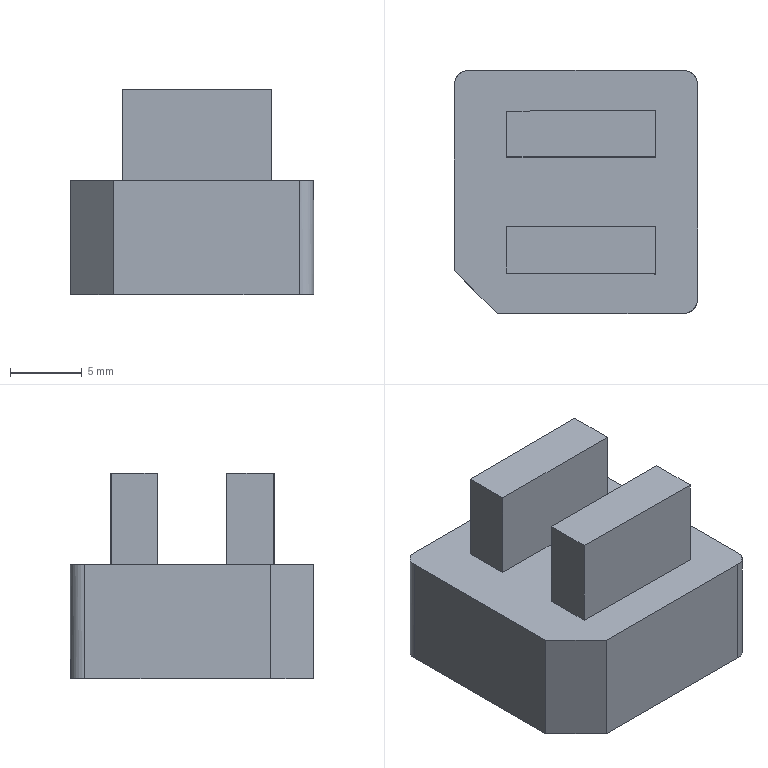NC program | PowerMill | posted with a generic post | part box 17 x 17 x 14.396 mm
Lines 1 to 1008 of 69084:
%
O0001
N104 ( POWERMILL CB  : 2026004.0)
N105 ( POST VER      : 2026.0.0.5161)
N106 ( OPTION FILE   : FANUC)
N107 ( OUTPUT WORKPLANE : WORLD)
N108 (  )
N109 ( TOOL LIST )
N110 (---------------------------------------)
N111 ( NO. | ID        | DIA.| TIP RAD|LENGTH)
N112 (---------------------------------------)
N113 (    1|D10C_1_1   |10.0 |  0.0   |69.84 )
N114 (   15|D3C_1_1    | 3.0 |  0.0   | 61.6 )
N115 (    3|D10_1_1    |10.0 |  0.0   |69.56 )
N116 (   10|D3_1_1     | 3.0 |  0.0   |61.56 )
N117 (   13|TEXT_D4_1_1| 4.0 |  0.3   |61.64 )
N118 (---------------------------------------)
N119 (  )
N120 ( NUMBER OF TOOLPATHS: 11.0 )
N121 ( ESTIMATED PROGRAM DURATION: 0 HOURS 10 MIN 28 SEC)
N122 (  )
N123 G00 G21 G80 G40 G17
N124 G90
N125 G54
N126 G53 Z0.0
N127 (---------------)
N128 ( START TOOLPATH : 精公开粗01-扫面平行-D10C )
N129 (---------------)
N130 ( TOOL NO.    :1 )
N131 ( TOOL TYPE   : ENDMILL)
N132 ( TOOL ID     : D10C_1_1)
N133 ( TOOL DIA    : 10.0 LENGTH 69.84)
N134 T1
N135 M6
N136 S8000 M03
N137 G00 G90 X0.0 Y0.0
N138 G43 Z10.2 H1
N139
N140 G05 P10000 R4
N141 X11.28 Y11.28
N142 Z1.126
N143 G01 Z-0.074 F6000.0
N144 X-11.28 F10000.0
N145 Y5.64
N146 X11.28
N147 Y0.0
N148 X-11.28
N149 Y-5.64
N150 X11.28
N151 Y-11.28
N152 X-11.28
N153 X-16.28
N154 G00 Z10.2
N155 G05 P0
N156 (---------------)
N157 ( END TOOLPATH : 精公开粗01-扫面平行-D10C )
N158 (---------------)
N159 ( START TOOLPATH : 精公开粗01-外形偏置-D10C )
N160 (---------------)
N161 G00 X0.3365 Y-0.0255 Z9.876
N162 G05 P10000 R4
N163 X-17.929 Y-10.5753
N164 Z0.6831
N165 G01 Z-0.5169 F6000.0
N166 X-17.4015 F10000.0
N167 G03 X-12.654 Y-5.8278 I0.0 J4.7475
N168 G01 Y12.468
N169 G02 X-11.654 Y13.468 I1.0 J0.0
N170 G01 X12.327
N171 G02 X13.327 Y12.468 I0.0 J-1.0
N172 G01 Y-12.519
N173 G02 X12.327 Y-13.519 I-1.0 J0.0
N174 G01 X-11.654
N175 G02 X-12.654 Y-12.519 I0.0 J1.0
N176 G01 Y-5.8278
N177 X-10.1543 Y-5.8262
N178 X-10.1562 Y-2.7325
N179 X-10.1353 Y-1.9591
N180 X-10.0077 Y-1.1856
N181 X-9.7559 Y-0.4122
N182 X-9.6387 Y-0.1635
N183 G03 X-9.6372 Y0.2593 I-0.4524 J0.213
N184 G01 X-9.6843 Y0.3612
N185 X-9.945 Y1.1346
N186 X-10.0804 Y1.9081
N187 X-10.1048 Y2.3039
N188 Y5.7609
N189 X-10.0266 Y6.5486
N190 X-9.8295 Y7.3221
N191 X-9.4981 Y8.0955
N192 X-9.3313 Y8.389
N193 X-9.0002 Y8.8689
N194 X-8.5579 Y9.3707
N195 X-8.2646 Y9.6423
N196 X-7.7845 Y10.0088
N197 X-7.0681 Y10.4158
N198 X-6.2376 Y10.7232
N199 X-5.4642 Y10.8766
N200 X-4.6908 Y10.9161
N201 X5.3638 Y10.9687
N202 X6.1372 Y10.9367
N203 X6.9106 Y10.7908
N204 X7.6841 Y10.5183
N205 X8.4575 Y10.0958
N206 X9.0488 Y9.6423
N207 X9.2309 Y9.4733
N208 X9.7637 Y8.8689
N209 X10.0043 Y8.5218
N210 X10.2482 Y8.0955
N211 X10.5695 Y7.3221
N212 X10.7578 Y6.5486
N213 X10.8275 Y5.7752
N214 X10.8281 Y2.6815
N215 X10.8024 Y1.9081
N216 X10.6669 Y1.1346
N217 X10.4063 Y0.3612
N218 X10.3359 Y0.2119
N219 G03 X10.3347 Y-0.2115 I0.4524 J-0.2131
N220 G01 X10.4278 Y-0.4122
N221 X10.6796 Y-1.1856
N222 X10.8072 Y-1.9591
N223 X10.8281 Y-2.7325
N224 X10.8274 Y-5.8262
N225 X10.7778 Y-6.4672
N226 X10.569 Y-7.3731
N227 X10.2476 Y-8.1465
N228 X10.0043 Y-8.5715
N229 X9.7627 Y-8.9199
N230 X9.2309 Y-9.523
N231 X9.0474 Y-9.6933
N232 X8.4575 Y-10.1455
N233 X7.8999 Y-10.4668
N234 X7.6841 Y-10.5681
N235 X6.9106 Y-10.8406
N236 X6.1372 Y-10.9864
N237 X5.3638 Y-11.0185
N238 X-4.6908 Y-10.9658
N239 X-5.4642 Y-10.932
N240 X-6.2376 Y-10.7863
N241 X-7.0111 Y-10.514
N242 X-7.7845 Y-10.0917
N243 X-8.3128 Y-9.6933
N244 X-8.5579 Y-9.4695
N245 X-9.0491 Y-8.9199
N246 X-9.3313 Y-8.5186
N247 X-9.5472 Y-8.1465
N248 X-9.8791 Y-7.3731
N249 X-10.0764 Y-6.5996
N250 X-10.1543 Y-5.8262
N251 X-12.654 Y-5.8278
N252 G00 Z3.2903
N253 G01 X-17.929 Y-10.5753
N254 G00 Z0.2903
N255 G01 Z-0.9097 F6000.0
N256 X-17.4015 F10000.0
N257 G03 X-12.654 Y-5.8278 I0.0 J4.7475
N258 G01 Y12.468
N259 G02 X-11.654 Y13.468 I1.0 J0.0
N260 G01 X12.327
N261 G02 X13.327 Y12.468 I0.0 J-1.0
N262 G01 Y-12.519
N263 G02 X12.327 Y-13.519 I-1.0 J0.0
N264 G01 X-11.654
N265 G02 X-12.654 Y-12.519 I0.0 J1.0
N266 G01 Y-5.8278
N267 X-10.1543 Y-5.8262
N268 X-10.1563 Y-2.7325
N269 X-10.1353 Y-1.9591
N270 X-10.0077 Y-1.1856
N271 X-9.7559 Y-0.4122
N272 X-9.6388 Y-0.1635
N273 G03 X-9.6372 Y0.2593 I-0.4523 J0.213
N274 G01 X-9.6843 Y0.3612
N275 X-9.945 Y1.1346
N276 X-10.0804 Y1.9081
N277 X-10.1048 Y2.3039
N278 Y5.7609
N279 X-10.0266 Y6.5486
N280 X-9.8296 Y7.3221
N281 X-9.4981 Y8.0955
N282 X-9.3313 Y8.389
N283 X-9.0002 Y8.8689
N284 X-8.5579 Y9.3707
N285 X-8.2646 Y9.6423
N286 X-7.7845 Y10.0088
N287 X-7.0681 Y10.4158
N288 X-6.2376 Y10.7232
N289 X-5.4642 Y10.8766
N290 X-4.6908 Y10.9161
N291 X5.3638 Y10.9687
N292 X6.1372 Y10.9367
N293 X6.9106 Y10.7908
N294 X7.6841 Y10.5183
N295 X8.4575 Y10.0958
N296 X9.0489 Y9.6423
N297 X9.2309 Y9.4733
N298 X9.7637 Y8.8689
N299 X10.0043 Y8.5218
N300 X10.2482 Y8.0955
N301 X10.5695 Y7.3221
N302 X10.7578 Y6.5486
N303 X10.8275 Y5.7752
N304 X10.8281 Y2.6815
N305 X10.8024 Y1.9081
N306 X10.6669 Y1.1346
N307 X10.4063 Y0.3612
N308 X10.3359 Y0.2119
N309 G03 X10.3347 Y-0.2116 I0.4524 J-0.2131
N310 G01 X10.4278 Y-0.4122
N311 X10.6796 Y-1.1856
N312 X10.8072 Y-1.9591
N313 X10.8281 Y-2.7325
N314 X10.8274 Y-5.8262
N315 X10.7778 Y-6.4672
N316 X10.569 Y-7.3731
N317 X10.2476 Y-8.1465
N318 X10.0043 Y-8.5715
N319 X9.7627 Y-8.9199
N320 X9.2309 Y-9.523
N321 X9.0474 Y-9.6933
N322 X8.4575 Y-10.1455
N323 X7.8999 Y-10.4668
N324 X7.6841 Y-10.5681
N325 X6.9106 Y-10.8406
N326 X6.1372 Y-10.9864
N327 X5.3638 Y-11.0185
N328 X-4.6908 Y-10.9658
N329 X-5.4642 Y-10.932
N330 X-6.2376 Y-10.7863
N331 X-7.0111 Y-10.514
N332 X-7.7845 Y-10.0917
N333 X-8.3128 Y-9.6933
N334 X-8.5579 Y-9.4695
N335 X-9.0491 Y-8.9199
N336 X-9.3313 Y-8.5186
N337 X-9.5472 Y-8.1465
N338 X-9.8791 Y-7.3731
N339 X-10.0764 Y-6.5996
N340 X-10.1543 Y-5.8262
N341 X-12.654 Y-5.8278
N342 G00 Z2.8974
N343 G01 X-17.929 Y-10.5753
N344 G00 Z-0.1026
N345 G01 Z-1.3026 F6000.0
N346 X-17.4015 F10000.0
N347 G03 X-12.654 Y-5.8278 I0.0 J4.7475
N348 G01 Y12.468
N349 G02 X-11.654 Y13.468 I1.0 J0.0
N350 G01 X12.327
N351 G02 X13.327 Y12.468 I0.0 J-1.0
N352 G01 Y-12.519
N353 G02 X12.327 Y-13.519 I-1.0 J0.0
N354 G01 X-11.654
N355 G02 X-12.654 Y-12.519 I0.0 J1.0
N356 G01 Y-5.8278
N357 X-10.1543 Y-5.8262
N358 X-10.1563 Y-2.7325
N359 X-10.1353 Y-1.9591
N360 X-10.0077 Y-1.1856
N361 X-9.7559 Y-0.4122
N362 X-9.6388 Y-0.1635
N363 G03 X-9.6372 Y0.2593 I-0.4523 J0.213
N364 G01 X-9.6844 Y0.3612
N365 X-9.945 Y1.1346
N366 X-10.0804 Y1.9081
N367 X-10.1048 Y2.3039
N368 Y5.7609
N369 X-10.0267 Y6.5486
N370 X-9.8296 Y7.3221
N371 X-9.4981 Y8.0955
N372 X-9.3313 Y8.389
N373 X-9.0002 Y8.8689
N374 X-8.5579 Y9.3707
N375 X-8.2646 Y9.6423
N376 X-7.7845 Y10.0088
N377 X-7.0681 Y10.4158
N378 X-6.2376 Y10.7232
N379 X-5.4642 Y10.8766
N380 X-4.6908 Y10.9161
N381 X5.3638 Y10.9687
N382 X6.1372 Y10.9367
N383 X6.9106 Y10.7908
N384 X7.6841 Y10.5183
N385 X8.4575 Y10.0958
N386 X9.0489 Y9.6423
N387 X9.2309 Y9.4733
N388 X9.7637 Y8.8689
N389 X10.0043 Y8.5218
N390 X10.2482 Y8.0955
N391 X10.5695 Y7.3221
N392 X10.7578 Y6.5486
N393 X10.8275 Y5.7752
N394 X10.8281 Y2.6815
N395 X10.8024 Y1.9081
N396 X10.6669 Y1.1346
N397 X10.4063 Y0.3612
N398 X10.336 Y0.2119
N399 G03 X10.3347 Y-0.2116 I0.4523 J-0.2131
N400 G01 X10.4278 Y-0.4122
N401 X10.6796 Y-1.1856
N402 X10.8072 Y-1.9591
N403 X10.8281 Y-2.7325
N404 X10.8274 Y-5.8262
N405 X10.7778 Y-6.4672
N406 X10.569 Y-7.3731
N407 X10.2476 Y-8.1465
N408 X10.0043 Y-8.5715
N409 X9.7627 Y-8.9199
N410 X9.2309 Y-9.523
N411 X9.0474 Y-9.6933
N412 X8.4575 Y-10.1455
N413 X7.8999 Y-10.4668
N414 X7.6841 Y-10.5681
N415 X6.9106 Y-10.8406
N416 X6.1372 Y-10.9864
N417 X5.3638 Y-11.0185
N418 X-4.6908 Y-10.9658
N419 X-5.4642 Y-10.932
N420 X-6.2376 Y-10.7863
N421 X-7.0111 Y-10.514
N422 X-7.7845 Y-10.0917
N423 X-8.3128 Y-9.6933
N424 X-8.5579 Y-9.4695
N425 X-9.0491 Y-8.9199
N426 X-9.3313 Y-8.5186
N427 X-9.5472 Y-8.1465
N428 X-9.8791 Y-7.3731
N429 X-10.0764 Y-6.5996
N430 X-10.1543 Y-5.8262
N431 X-12.654 Y-5.8278
N432 G00 Z2.5045
N433 G01 X-17.929 Y-10.5753
N434 G00 Z-0.4955
N435 G01 Z-1.6955 F6000.0
N436 X-17.4015 F10000.0
N437 G03 X-12.654 Y-5.8278 I0.0 J4.7475
N438 G01 Y12.468
N439 G02 X-11.654 Y13.468 I1.0 J0.0
N440 G01 X12.327
N441 G02 X13.327 Y12.468 I0.0 J-1.0
N442 G01 Y-12.519
N443 G02 X12.327 Y-13.519 I-1.0 J0.0
N444 G01 X-11.654
N445 G02 X-12.654 Y-12.519 I0.0 J1.0
N446 G01 Y-5.8278
N447 X-10.1543 Y-5.8262
N448 X-10.1563 Y-2.7325
N449 X-10.1353 Y-1.9591
N450 X-10.0077 Y-1.1856
N451 X-9.7559 Y-0.4122
N452 X-9.6388 Y-0.1635
N453 G03 X-9.6372 Y0.2593 I-0.4523 J0.213
N454 G01 X-9.6844 Y0.3612
N455 X-9.945 Y1.1346
N456 X-10.0804 Y1.9081
N457 X-10.1048 Y2.3039
N458 Y5.7609
N459 X-10.0267 Y6.5486
N460 X-9.8296 Y7.3221
N461 X-9.4981 Y8.0955
N462 X-9.3313 Y8.389
N463 X-9.0002 Y8.8689
N464 X-8.5579 Y9.3707
N465 X-8.2646 Y9.6423
N466 X-7.7845 Y10.0088
N467 X-7.0681 Y10.4158
N468 X-6.2376 Y10.7232
N469 X-5.4642 Y10.8767
N470 X-4.6908 Y10.9161
N471 X5.3638 Y10.9687
N472 X6.1372 Y10.9367
N473 X6.9106 Y10.7908
N474 X7.6841 Y10.5183
N475 X8.4575 Y10.0958
N476 X9.0489 Y9.6423
N477 X9.2309 Y9.4733
N478 X9.7637 Y8.8689
N479 X10.0043 Y8.5218
N480 X10.2482 Y8.0955
N481 X10.5695 Y7.3221
N482 X10.7578 Y6.5486
N483 X10.8275 Y5.7752
N484 X10.8281 Y2.6815
N485 X10.8024 Y1.9081
N486 X10.667 Y1.1346
N487 X10.4063 Y0.3612
N488 X10.336 Y0.2119
N489 G03 X10.3347 Y-0.2116 I0.4523 J-0.2131
N490 G01 X10.4278 Y-0.4122
N491 X10.6796 Y-1.1856
N492 X10.8072 Y-1.9591
N493 X10.8281 Y-2.7325
N494 X10.8274 Y-5.8262
N495 X10.7778 Y-6.4672
N496 X10.569 Y-7.3731
N497 X10.2476 Y-8.1465
N498 X10.0043 Y-8.5715
N499 X9.7627 Y-8.9199
N500 X9.2309 Y-9.523
N501 X9.0475 Y-9.6933
N502 X8.4575 Y-10.1456
N503 X7.8999 Y-10.4668
N504 X7.6841 Y-10.5681
N505 X6.9106 Y-10.8406
N506 X6.1372 Y-10.9864
N507 X5.3638 Y-11.0185
N508 X-4.6908 Y-10.9658
N509 X-5.4642 Y-10.932
N510 X-6.2376 Y-10.7863
N511 X-7.0111 Y-10.514
N512 X-7.7845 Y-10.0917
N513 X-8.3128 Y-9.6933
N514 X-8.5579 Y-9.4695
N515 X-9.0491 Y-8.9199
N516 X-9.3313 Y-8.5187
N517 X-9.5472 Y-8.1465
N518 X-9.8791 Y-7.3731
N519 X-10.0764 Y-6.5996
N520 X-10.1543 Y-5.8262
N521 X-12.654 Y-5.8278
N522 G00 Z2.1116
N523 G01 X-17.929 Y-10.5753
N524 G00 Z-0.8884
N525 G01 Z-2.0884 F6000.0
N526 X-17.4015 F10000.0
N527 G03 X-12.654 Y-5.8278 I0.0 J4.7475
N528 G01 Y12.468
N529 G02 X-11.654 Y13.468 I1.0 J0.0
N530 G01 X12.327
N531 G02 X13.327 Y12.468 I0.0 J-1.0
N532 G01 Y-12.519
N533 G02 X12.327 Y-13.519 I-1.0 J0.0
N534 G01 X-11.654
N535 G02 X-12.654 Y-12.519 I0.0 J1.0
N536 G01 Y-5.8278
N537 X-10.1543 Y-5.8262
N538 X-10.1563 Y-2.7325
N539 X-10.1353 Y-1.9591
N540 X-10.0077 Y-1.1856
N541 X-9.7559 Y-0.4122
N542 X-9.6388 Y-0.1635
N543 G03 X-9.6372 Y0.2593 I-0.4523 J0.213
N544 G01 X-9.6844 Y0.3612
N545 X-9.945 Y1.1346
N546 X-10.0804 Y1.9081
N547 X-10.1048 Y2.3038
N548 Y5.7609
N549 X-10.0267 Y6.5486
N550 X-9.8296 Y7.3221
N551 X-9.4981 Y8.0955
N552 X-9.3313 Y8.389
N553 X-9.0002 Y8.8689
N554 X-8.5579 Y9.3707
N555 X-8.2646 Y9.6423
N556 X-7.7845 Y10.0088
N557 X-7.0681 Y10.4158
N558 X-6.2376 Y10.7232
N559 X-5.4642 Y10.8767
N560 X-4.6908 Y10.9161
N561 X5.3638 Y10.9687
N562 X6.1372 Y10.9367
N563 X6.9106 Y10.7908
N564 X7.6841 Y10.5183
N565 X8.4575 Y10.0958
N566 X9.0489 Y9.6423
N567 X9.2309 Y9.4733
N568 X9.7637 Y8.8689
N569 X10.0043 Y8.5218
N570 X10.2482 Y8.0955
N571 X10.5695 Y7.3221
N572 X10.7578 Y6.5486
N573 X10.8275 Y5.7752
N574 X10.8281 Y2.6815
N575 X10.8024 Y1.9081
N576 X10.667 Y1.1346
N577 X10.4063 Y0.3612
N578 X10.336 Y0.2119
N579 G03 X10.3347 Y-0.2116 I0.4523 J-0.2131
N580 G01 X10.4278 Y-0.4122
N581 X10.6796 Y-1.1856
N582 X10.8072 Y-1.9591
N583 X10.8281 Y-2.7325
N584 X10.8274 Y-5.8262
N585 X10.7778 Y-6.4672
N586 X10.569 Y-7.3731
N587 X10.2476 Y-8.1465
N588 X10.0043 Y-8.5715
N589 X9.7627 Y-8.9199
N590 X9.2309 Y-9.523
N591 X9.0475 Y-9.6933
N592 X8.4575 Y-10.1456
N593 X7.8999 Y-10.4668
N594 X7.6841 Y-10.5681
N595 X6.9106 Y-10.8406
N596 X6.1372 Y-10.9864
N597 X5.3638 Y-11.0185
N598 X-4.6908 Y-10.9658
N599 X-5.4642 Y-10.932
N600 X-6.2376 Y-10.7863
N601 X-7.0111 Y-10.514
N602 X-7.7845 Y-10.0917
N603 X-8.3128 Y-9.6933
N604 X-8.5579 Y-9.4695
N605 X-9.0491 Y-8.9199
N606 X-9.3313 Y-8.5187
N607 X-9.5472 Y-8.1465
N608 X-9.8791 Y-7.3731
N609 X-10.0764 Y-6.5996
N610 X-10.1543 Y-5.8262
N611 X-12.654 Y-5.8278
N612 G00 Z1.7188
N613 G01 X-17.929 Y-10.5753
N614 G00 Z-1.2813
N615 G01 Z-2.4813 F6000.0
N616 X-17.4015 F10000.0
N617 G03 X-12.654 Y-5.8278 I0.0 J4.7475
N618 G01 Y12.468
N619 G02 X-11.654 Y13.468 I1.0 J0.0
N620 G01 X12.327
N621 G02 X13.327 Y12.468 I0.0 J-1.0
N622 G01 Y-12.519
N623 G02 X12.327 Y-13.519 I-1.0 J0.0
N624 G01 X-11.654
N625 G02 X-12.654 Y-12.519 I0.0 J1.0
N626 G01 Y-5.8278
N627 X-10.1543 Y-5.8262
N628 X-10.1563 Y-2.7325
N629 X-10.1353 Y-1.9591
N630 X-10.0077 Y-1.1856
N631 X-9.7559 Y-0.4122
N632 X-9.6388 Y-0.1635
N633 G03 X-9.6373 Y0.2593 I-0.4523 J0.213
N634 G01 X-9.6844 Y0.3612
N635 X-9.945 Y1.1346
N636 X-10.0804 Y1.9081
N637 X-10.1048 Y2.3038
N638 Y5.7609
N639 X-10.0267 Y6.5486
N640 X-9.8296 Y7.3221
N641 X-9.4981 Y8.0955
N642 X-9.3313 Y8.389
N643 X-9.0002 Y8.8689
N644 X-8.5579 Y9.3707
N645 X-8.2646 Y9.6423
N646 X-7.7845 Y10.0088
N647 X-7.0681 Y10.4158
N648 X-6.2376 Y10.7232
N649 X-5.4642 Y10.8767
N650 X-4.6908 Y10.9161
N651 X5.3638 Y10.9688
N652 X6.1372 Y10.9367
N653 X6.9106 Y10.7908
N654 X7.6841 Y10.5183
N655 X8.4575 Y10.0958
N656 X9.0489 Y9.6423
N657 X9.2309 Y9.4733
N658 X9.7637 Y8.8689
N659 X10.0043 Y8.5218
N660 X10.2483 Y8.0955
N661 X10.5695 Y7.3221
N662 X10.7578 Y6.5486
N663 X10.8275 Y5.7752
N664 X10.8282 Y2.6815
N665 X10.8024 Y1.9081
N666 X10.667 Y1.1346
N667 X10.4063 Y0.3612
N668 X10.336 Y0.2119
N669 G03 X10.3347 Y-0.2116 I0.4523 J-0.2131
N670 G01 X10.4278 Y-0.4122
N671 X10.6797 Y-1.1856
N672 X10.8072 Y-1.9591
N673 X10.8282 Y-2.7325
N674 X10.8274 Y-5.8262
N675 X10.7778 Y-6.4672
N676 X10.569 Y-7.3731
N677 X10.2476 Y-8.1465
N678 X10.0043 Y-8.5716
N679 X9.7627 Y-8.9199
N680 X9.2309 Y-9.523
N681 X9.0475 Y-9.6933
N682 X8.4575 Y-10.1456
N683 X7.8999 Y-10.4668
N684 X7.6841 Y-10.5681
N685 X6.9106 Y-10.8406
N686 X6.1372 Y-10.9864
N687 X5.3638 Y-11.0185
N688 X-4.6908 Y-10.9658
N689 X-5.4642 Y-10.932
N690 X-6.2376 Y-10.7863
N691 X-7.0111 Y-10.514
N692 X-7.7845 Y-10.0917
N693 X-8.3128 Y-9.6933
N694 X-8.5579 Y-9.4695
N695 X-9.0491 Y-8.9199
N696 X-9.3313 Y-8.5187
N697 X-9.5472 Y-8.1465
N698 X-9.8791 Y-7.3731
N699 X-10.0764 Y-6.5996
N700 X-10.1543 Y-5.8262
N701 X-12.654 Y-5.8278
N702 G00 Z1.3259
N703 G01 X-17.929 Y-10.5753
N704 G00 Z-1.6741
N705 G01 Z-2.8741 F6000.0
N706 X-17.4015 F10000.0
N707 G03 X-12.654 Y-5.8278 I0.0 J4.7475
N708 G01 Y12.468
N709 G02 X-11.654 Y13.468 I1.0 J0.0
N710 G01 X12.327
N711 G02 X13.327 Y12.468 I0.0 J-1.0
N712 G01 Y-12.519
N713 G02 X12.327 Y-13.519 I-1.0 J0.0
N714 G01 X-11.654
N715 G02 X-12.654 Y-12.519 I0.0 J1.0
N716 G01 Y-5.8278
N717 X-10.1543 Y-5.8262
N718 X-10.1563 Y-2.7325
N719 X-10.1353 Y-1.9591
N720 X-10.0077 Y-1.1856
N721 X-9.7559 Y-0.4122
N722 X-9.6388 Y-0.1635
N723 G03 X-9.6373 Y0.2593 I-0.4523 J0.213
N724 G01 X-9.6844 Y0.3612
N725 X-9.945 Y1.1346
N726 X-10.0804 Y1.9081
N727 X-10.1048 Y2.3038
N728 Y5.7609
N729 X-10.0267 Y6.5486
N730 X-9.8296 Y7.3221
N731 X-9.4981 Y8.0955
N732 X-9.3313 Y8.389
N733 X-9.0002 Y8.8689
N734 X-8.5579 Y9.3708
N735 X-8.2646 Y9.6423
N736 X-7.7845 Y10.0088
N737 X-7.0681 Y10.4158
N738 X-6.2376 Y10.7232
N739 X-5.4642 Y10.8767
N740 X-4.6908 Y10.9161
N741 X5.3638 Y10.9688
N742 X6.1372 Y10.9367
N743 X6.9106 Y10.7908
N744 X7.6841 Y10.5183
N745 X8.4575 Y10.0958
N746 X9.0489 Y9.6423
N747 X9.2309 Y9.4733
N748 X9.7637 Y8.8689
N749 X10.0043 Y8.5218
N750 X10.2483 Y8.0955
N751 X10.5695 Y7.3221
N752 X10.7579 Y6.5486
N753 X10.8275 Y5.7752
N754 X10.8282 Y2.6815
N755 X10.8024 Y1.9081
N756 X10.667 Y1.1346
N757 X10.4063 Y0.3612
N758 X10.336 Y0.212
N759 G03 X10.3347 Y-0.2116 I0.4523 J-0.2132
N760 G01 X10.4278 Y-0.4122
N761 X10.6797 Y-1.1856
N762 X10.8072 Y-1.9591
N763 X10.8282 Y-2.7325
N764 X10.8274 Y-5.8262
N765 X10.7778 Y-6.4672
N766 X10.569 Y-7.3731
N767 X10.2476 Y-8.1465
N768 X10.0043 Y-8.5716
N769 X9.7627 Y-8.9199
N770 X9.2309 Y-9.523
N771 X9.0475 Y-9.6933
N772 X8.4575 Y-10.1456
N773 X7.8999 Y-10.4668
N774 X7.6841 Y-10.5681
N775 X6.9106 Y-10.8406
N776 X6.1372 Y-10.9864
N777 X5.3638 Y-11.0185
N778 X-4.6908 Y-10.9658
N779 X-5.4642 Y-10.932
N780 X-6.2376 Y-10.7863
N781 X-7.0111 Y-10.514
N782 X-7.7845 Y-10.0917
N783 X-8.3128 Y-9.6933
N784 X-8.5579 Y-9.4695
N785 X-9.0491 Y-8.9199
N786 X-9.3313 Y-8.5187
N787 X-9.5472 Y-8.1465
N788 X-9.8791 Y-7.3731
N789 X-10.0764 Y-6.5996
N790 X-10.1543 Y-5.8262
N791 X-12.654 Y-5.8278
N792 G00 Z0.933
N793 G01 X-17.929 Y-10.5753
N794 G00 Z-2.067
N795 G01 Z-3.267 F6000.0
N796 X-17.4015 F10000.0
N797 G03 X-12.654 Y-5.8278 I0.0 J4.7475
N798 G01 Y12.468
N799 G02 X-11.654 Y13.468 I1.0 J0.0
N800 G01 X12.327
N801 G02 X13.327 Y12.468 I0.0 J-1.0
N802 G01 Y-12.519
N803 G02 X12.327 Y-13.519 I-1.0 J0.0
N804 G01 X-11.654
N805 G02 X-12.654 Y-12.519 I0.0 J1.0
N806 G01 Y-5.8278
N807 X-10.1543 Y-5.8262
N808 X-10.1563 Y-2.7325
N809 X-10.1353 Y-1.9591
N810 X-10.0077 Y-1.1856
N811 X-9.7559 Y-0.4122
N812 X-9.6388 Y-0.1635
N813 G03 X-9.6373 Y0.2593 I-0.4523 J0.213
N814 G01 X-9.6844 Y0.3612
N815 X-9.945 Y1.1346
N816 X-10.0804 Y1.9081
N817 X-10.1048 Y2.3038
N818 Y5.7609
N819 X-10.0267 Y6.5486
N820 X-9.8296 Y7.3221
N821 X-9.4981 Y8.0955
N822 X-9.3313 Y8.389
N823 X-9.0002 Y8.8689
N824 X-8.5579 Y9.3708
N825 X-8.2646 Y9.6423
N826 X-7.7845 Y10.0088
N827 X-7.0681 Y10.4158
N828 X-6.2376 Y10.7232
N829 X-5.4642 Y10.8767
N830 X-4.6908 Y10.9162
N831 X5.3638 Y10.9688
N832 X6.1372 Y10.9367
N833 X6.9106 Y10.7908
N834 X7.6841 Y10.5184
N835 X8.4575 Y10.0958
N836 X9.0489 Y9.6423
N837 X9.2309 Y9.4733
N838 X9.7637 Y8.8689
N839 X10.0043 Y8.5218
N840 X10.2483 Y8.0955
N841 X10.5695 Y7.3221
N842 X10.7579 Y6.5486
N843 X10.8275 Y5.7752
N844 X10.8282 Y2.6815
N845 X10.8024 Y1.9081
N846 X10.667 Y1.1346
N847 X10.4063 Y0.3612
N848 X10.336 Y0.212
N849 G03 X10.3347 Y-0.2116 I0.4523 J-0.2132
N850 G01 X10.4278 Y-0.4122
N851 X10.6797 Y-1.1856
N852 X10.8072 Y-1.9591
N853 X10.8282 Y-2.7325
N854 X10.8274 Y-5.8262
N855 X10.7778 Y-6.4672
N856 X10.569 Y-7.3731
N857 X10.2476 Y-8.1465
N858 X10.0043 Y-8.5716
N859 X9.7627 Y-8.9199
N860 X9.2309 Y-9.523
N861 X9.0475 Y-9.6933
N862 X8.4575 Y-10.1456
N863 X7.8999 Y-10.4668
N864 X7.6841 Y-10.5681
N865 X6.9106 Y-10.8406
N866 X6.1372 Y-10.9864
N867 X5.3638 Y-11.0185
N868 X-4.6908 Y-10.9658
N869 X-5.4642 Y-10.932
N870 X-6.2376 Y-10.7863
N871 X-7.0111 Y-10.514
N872 X-7.7845 Y-10.0917
N873 X-8.3128 Y-9.6933
N874 X-8.5579 Y-9.4695
N875 X-9.0491 Y-8.9199
N876 X-9.3313 Y-8.5187
N877 X-9.5473 Y-8.1465
N878 X-9.8791 Y-7.3731
N879 X-10.0764 Y-6.5996
N880 X-10.1543 Y-5.8262
N881 X-12.654 Y-5.8278
N882 G00 Z0.5401
N883 G01 X-17.929 Y-10.5753
N884 G00 Z-2.4599
N885 G01 Z-3.6599 F6000.0
N886 X-17.4015 F10000.0
N887 G03 X-12.654 Y-5.8278 I0.0 J4.7475
N888 G01 Y12.468
N889 G02 X-11.654 Y13.468 I1.0 J0.0
N890 G01 X12.327
N891 G02 X13.327 Y12.468 I0.0 J-1.0
N892 G01 Y-12.519
N893 G02 X12.327 Y-13.519 I-1.0 J0.0
N894 G01 X-11.654
N895 G02 X-12.654 Y-12.519 I0.0 J1.0
N896 G01 Y-5.8278
N897 X-10.1543 Y-5.8262
N898 X-10.1563 Y-2.7325
N899 X-10.1353 Y-1.9591
N900 X-10.0077 Y-1.1856
N901 X-9.7559 Y-0.4122
N902 X-9.6388 Y-0.1635
N903 G03 X-9.6373 Y0.2593 I-0.4523 J0.213
N904 G01 X-9.6844 Y0.3612
N905 X-9.945 Y1.1346
N906 X-10.0804 Y1.9081
N907 X-10.1048 Y2.3038
N908 Y5.7609
N909 X-10.0267 Y6.5486
N910 X-9.8296 Y7.3221
N911 X-9.4981 Y8.0955
N912 X-9.3313 Y8.389
N913 X-9.0003 Y8.8689
N914 X-8.5579 Y9.3708
N915 X-8.2646 Y9.6423
N916 X-7.7845 Y10.0088
N917 X-7.0682 Y10.4158
N918 X-6.2376 Y10.7232
N919 X-5.4642 Y10.8767
N920 X-4.6908 Y10.9162
N921 X5.3638 Y10.9688
N922 X6.1372 Y10.9368
N923 X6.9106 Y10.7908
N924 X7.6841 Y10.5184
N925 X8.4575 Y10.0958
N926 X9.0489 Y9.6423
N927 X9.2309 Y9.4733
N928 X9.7637 Y8.8689
N929 X10.0043 Y8.5218
N930 X10.2483 Y8.0955
N931 X10.5695 Y7.3221
N932 X10.7579 Y6.5486
N933 X10.8275 Y5.7752
N934 X10.8282 Y2.6815
N935 X10.8024 Y1.9081
N936 X10.667 Y1.1346
N937 X10.4063 Y0.3612
N938 X10.336 Y0.212
N939 G03 X10.3347 Y-0.2116 I0.4523 J-0.2132
N940 G01 X10.4278 Y-0.4122
N941 X10.6797 Y-1.1856
N942 X10.8072 Y-1.9591
N943 X10.8282 Y-2.7325
N944 X10.8274 Y-5.8262
N945 X10.7778 Y-6.4672
N946 X10.569 Y-7.3731
N947 X10.2476 Y-8.1465
N948 X10.0043 Y-8.5716
N949 X9.7627 Y-8.9199
N950 X9.2309 Y-9.523
N951 X9.0475 Y-9.6933
N952 X8.4575 Y-10.1456
N953 X7.8999 Y-10.4668
N954 X7.6841 Y-10.5681
N955 X6.9106 Y-10.8406
N956 X6.1372 Y-10.9864
N957 X5.3638 Y-11.0185
N958 X-4.6908 Y-10.9658
N959 X-5.4642 Y-10.932
N960 X-6.2376 Y-10.7863
N961 X-7.0111 Y-10.514
N962 X-7.7845 Y-10.0918
N963 X-8.3128 Y-9.6933
N964 X-8.5579 Y-9.4696
N965 X-9.0491 Y-8.9199
N966 X-9.3313 Y-8.5187
N967 X-9.5473 Y-8.1465
N968 X-9.8791 Y-7.3731
N969 X-10.0764 Y-6.5996
N970 X-10.1543 Y-5.8262
N971 X-12.654 Y-5.8278
N972 G00 Z0.1472
N973 G01 X-17.929 Y-10.5753
N974 G00 Z-2.8528
N975 G01 Z-4.0528 F6000.0
N976 X-17.4015 F10000.0
N977 G03 X-12.654 Y-5.8278 I0.0 J4.7475
N978 G01 Y12.468
N979 G02 X-11.654 Y13.468 I1.0 J0.0
N980 G01 X12.327
N981 G02 X13.327 Y12.468 I0.0 J-1.0
N982 G01 Y-12.519
N983 G02 X12.327 Y-13.519 I-1.0 J0.0
N984 G01 X-11.654
N985 G02 X-12.654 Y-12.519 I0.0 J1.0
N986 G01 Y-5.8278
N987 X-10.1543 Y-5.8262
N988 X-10.1563 Y-2.7325
N989 X-10.1353 Y-1.9591
N990 X-10.0077 Y-1.1856
N991 X-9.7559 Y-0.4122
N992 X-9.6388 Y-0.1635
N993 G03 X-9.6373 Y0.2593 I-0.4523 J0.213
N994 G01 X-9.6844 Y0.3612
N995 X-9.945 Y1.1346
N996 X-10.0805 Y1.9081
N997 X-10.1048 Y2.3038
N998 Y5.7609
N999 X-10.0267 Y6.5486
N1000 X-9.8296 Y7.3221
N1001 X-9.4981 Y8.0955
N1002 X-9.3313 Y8.389
N1003 X-9.0003 Y8.8689
N1004 X-8.5579 Y9.3708
N1005 X-8.2646 Y9.6423
N1006 X-7.7845 Y10.0088
N1007 X-7.0682 Y10.4158
N1008 X-6.2376 Y10.7232
N1009 X-5.4642 Y10.8767
N1010 X-4.6908 Y10.9162
N1011 X5.3638 Y10.9688
N1012 X6.1372 Y10.9368
N1013 X6.9106 Y10.7908
N1014 X7.6841 Y10.5184
N1015 X8.4575 Y10.0958
N1016 X9.0489 Y9.6423
N1017 X9.2309 Y9.4733
N1018 X9.7637 Y8.8689
N1019 X10.0043 Y8.5218
N1020 X10.2483 Y8.0955
N1021 X10.5695 Y7.3221
N1022 X10.7579 Y6.5486
N1023 X10.8275 Y5.7752
N1024 X10.8282 Y2.6815
N1025 X10.8024 Y1.9081
N1026 X10.667 Y1.1346
N1027 X10.4063 Y0.3612
N1028 X10.336 Y0.212
N1029 G03 X10.3347 Y-0.2116 I0.4523 J-0.2132
N1030 G01 X10.4278 Y-0.4122
N1031 X10.6797 Y-1.1856
N1032 X10.8072 Y-1.9591
N1033 X10.8282 Y-2.7325
N1034 X10.8274 Y-5.8262
N1035 X10.7778 Y-6.4673
N1036 X10.5691 Y-7.3731
N1037 X10.2476 Y-8.1465
N1038 X10.0043 Y-8.5716
N1039 X9.7627 Y-8.9199
N1040 X9.2309 Y-9.523
N1041 X9.0475 Y-9.6933
N1042 X8.4575 Y-10.1456
N1043 X7.8999 Y-10.4668
N1044 X7.6841 Y-10.5681
N1045 X6.9106 Y-10.8406
N1046 X6.1372 Y-10.9864
N1047 X5.3638 Y-11.0185
N1048 X-4.6908 Y-10.9658
N1049 X-5.4642 Y-10.932
N1050 X-6.2376 Y-10.7863
N1051 X-7.0111 Y-10.514
N1052 X-7.7845 Y-10.0918
N1053 X-8.3128 Y-9.6933
N1054 X-8.5579 Y-9.4696
N1055 X-9.0491 Y-8.9199
N1056 X-9.3313 Y-8.5187
N1057 X-9.5473 Y-8.1465
N1058 X-9.8791 Y-7.3731
N1059 X-10.0764 Y-6.5996
N1060 X-10.1543 Y-5.8262
N1061 X-12.654 Y-5.8278
N1062 G00 Z-0.2456
N1063 G01 X-17.929 Y-10.5753
N1064 G00 Z-3.2456
N1065 G01 Z-4.4456 F6000.0
N1066 X-17.4015 F10000.0
N1067 G03 X-12.654 Y-5.8278 I0.0 J4.7475
N1068 G01 Y12.468
N1069 G02 X-11.654 Y13.468 I1.0 J0.0
N1070 G01 X12.327
N1071 G02 X13.327 Y12.468 I0.0 J-1.0
N1072 G01 Y-12.519
N1073 G02 X12.327 Y-13.519 I-1.0 J0.0
N1074 G01 X-11.654
N1075 G02 X-12.654 Y-12.519 I0.0 J1.0
N1076 G01 Y-5.8278
N1077 X-10.1543 Y-5.8262
N1078 X-10.1563 Y-2.7325
N1079 X-10.1353 Y-1.9591
N1080 X-10.0077 Y-1.1856
N1081 X-9.7559 Y-0.4122
N1082 X-9.6388 Y-0.1636
N1083 G03 X-9.6373 Y0.2593 I-0.4523 J0.2131
N1084 G01 X-9.6844 Y0.3612
N1085 X-9.945 Y1.1346
N1086 X-10.0805 Y1.9081
N1087 X-10.1048 Y2.3038
N1088 Y5.7609
N1089 X-10.0267 Y6.5486
N1090 X-9.8296 Y7.3221
N1091 X-9.4981 Y8.0955
N1092 X-9.3313 Y8.389
N1093 X-9.0003 Y8.8689
N1094 X-8.5579 Y9.3708
N1095 X-8.2646 Y9.6423
N1096 X-7.7845 Y10.0088
N1097 X-7.0682 Y10.4158
N1098 X-6.2376 Y10.7232
N1099 X-5.4642 Y10.8767
N1100 X-4.6908 Y10.9162
N1101 X5.3638 Y10.9688
N1102 X6.1372 Y10.9368
N1103 X6.9106 Y10.7908
N1104 X7.6841 Y10.5184
N1105 X8.4575 Y10.0958